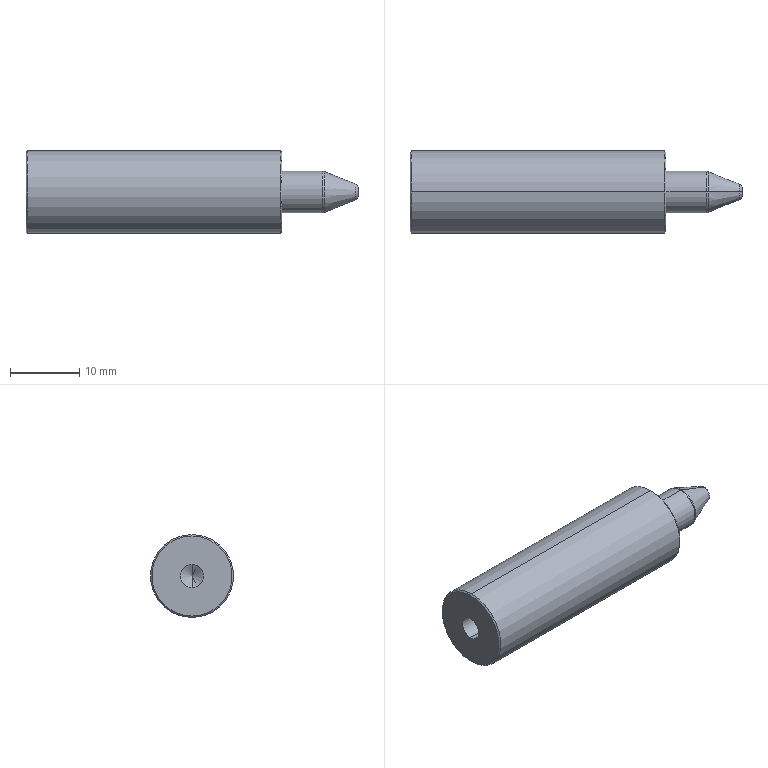Part | STEP file | 1 solid | 21 faces | box 48 x 12 x 12 mm | volume 4302 mm3 | cone 8 | cylinder 6 | torus 4 | plane 3 | commonest cylinder face diameters 3.3 x2 6 x2 12 x2
STEP:
#1=CARTESIAN_POINT('',(0.,0.,0.));
#2=DIRECTION('',(0.,0.,1.));
#3=DIRECTION('',(1.,0.,0.));
#4=AXIS2_PLACEMENT_3D('',#1,#2,#3);
#5=CARTESIAN_POINT('',(42.904,0.,3.));
#6=VERTEX_POINT('',#5);
#7=CARTESIAN_POINT('',(42.904,0.,-3.));
#8=VERTEX_POINT('',#7);
#9=CARTESIAN_POINT('',(42.904,0.,0.));
#10=DIRECTION('',(-1.,0.,0.));
#11=DIRECTION('',(0.,0.,-1.));
#12=AXIS2_PLACEMENT_3D('',#9,#10,#11);
#13=CIRCLE('',#12,3.);
#14=CARTESIAN_POINT('',(42.904,0.,0.));
#15=DIRECTION('',(1.,0.,0.));
#16=DIRECTION('',(0.,0.,-1.));
#17=AXIS2_PLACEMENT_3D('',#14,#15,#16);
#18=TOROIDAL_SURFACE('',#17,2.5,0.5);
#19=CARTESIAN_POINT('',(6.283,0.));
#20=DIRECTION('',(-1.,0.));
#21=VECTOR('',#20,1.);
#22=LINE('',#19,#21);
#23=(GEOMETRIC_REPRESENTATION_CONTEXT(2)PARAMETRIC_REPRESENTATION_CONTEXT()REPRESENTATION_CONTEXT('',''));
#24=DEFINITIONAL_REPRESENTATION('',(#22),#23);
#25=PCURVE('',#18,#24);
#26=CARTESIAN_POINT('',(0.,0.,0.));
#27=DIRECTION('',(-1.,0.,0.));
#28=DIRECTION('',(0.,0.,1.));
#29=AXIS2_PLACEMENT_3D('',#26,#27,#28);
#30=CYLINDRICAL_SURFACE('',#29,3.);
#31=CARTESIAN_POINT('',(-3.142,-42.904));
#32=DIRECTION('',(1.,0.));
#33=VECTOR('',#32,1.);
#34=LINE('',#31,#33);
#35=(GEOMETRIC_REPRESENTATION_CONTEXT(2)PARAMETRIC_REPRESENTATION_CONTEXT()REPRESENTATION_CONTEXT('',''));
#36=DEFINITIONAL_REPRESENTATION('',(#34),#35);
#37=PCURVE('',#30,#36);
#38=SURFACE_CURVE('',#13,(#25,#37),.PCURVE_S1.);
#39=EDGE_CURVE('',#6,#8,#38,.T.);
#40=ORIENTED_EDGE('',*,*,#39,.F.);
#41=CARTESIAN_POINT('',(43.089,0.,2.964));
#42=VERTEX_POINT('',#41);
#43=CARTESIAN_POINT('',(42.904,0.,2.5));
#44=DIRECTION('',(0.,1.,0.));
#45=DIRECTION('',(0.,0.,1.));
#46=AXIS2_PLACEMENT_3D('',#43,#44,#45);
#47=CIRCLE('',#46,0.5);
#48=CARTESIAN_POINT('',(3.142,0.));
#49=DIRECTION('',(0.,1.));
#50=VECTOR('',#49,1.);
#51=LINE('',#48,#50);
#52=(GEOMETRIC_REPRESENTATION_CONTEXT(2)PARAMETRIC_REPRESENTATION_CONTEXT()REPRESENTATION_CONTEXT('',''));
#53=DEFINITIONAL_REPRESENTATION('',(#51),#52);
#54=PCURVE('',#18,#53);
#55=CARTESIAN_POINT('',(42.904,0.,0.));
#56=DIRECTION('',(1.,0.,0.));
#57=DIRECTION('',(0.,0.,-1.));
#58=AXIS2_PLACEMENT_3D('',#55,#56,#57);
#59=TOROIDAL_SURFACE('',#58,2.5,0.5);
#60=CARTESIAN_POINT('',(3.142,0.));
#61=DIRECTION('',(0.,1.));
#62=VECTOR('',#61,1.);
#63=LINE('',#60,#62);
#64=(GEOMETRIC_REPRESENTATION_CONTEXT(2)PARAMETRIC_REPRESENTATION_CONTEXT()REPRESENTATION_CONTEXT('',''));
#65=DEFINITIONAL_REPRESENTATION('',(#63),#64);
#66=PCURVE('',#59,#65);
#67=SURFACE_CURVE('',#47,(#54,#66),.PCURVE_S1.);
#68=EDGE_CURVE('',#6,#42,#67,.T.);
#69=ORIENTED_EDGE('',*,*,#68,.T.);
#70=CARTESIAN_POINT('',(43.089,0.,-2.964));
#71=VERTEX_POINT('',#70);
#72=CARTESIAN_POINT('',(43.089,0.,0.));
#73=DIRECTION('',(1.,0.,0.));
#74=DIRECTION('',(0.,0.,1.));
#75=AXIS2_PLACEMENT_3D('',#72,#73,#74);
#76=CIRCLE('',#75,2.964);
#77=CARTESIAN_POINT('',(-3.142,0.3805));
#78=DIRECTION('',(1.,0.));
#79=VECTOR('',#78,1.);
#80=LINE('',#77,#79);
#81=(GEOMETRIC_REPRESENTATION_CONTEXT(2)PARAMETRIC_REPRESENTATION_CONTEXT()REPRESENTATION_CONTEXT('',''));
#82=DEFINITIONAL_REPRESENTATION('',(#80),#81);
#83=PCURVE('',#18,#82);
#84=CARTESIAN_POINT('',(43.,0.,0.));
#85=DIRECTION('',(-1.,0.,0.));
#86=DIRECTION('',(0.,0.,1.));
#87=AXIS2_PLACEMENT_3D('',#84,#85,#86);
#88=CONICAL_SURFACE('',#87,3.,0.3805);
#89=CARTESIAN_POINT('',(6.283,-0.0894));
#90=DIRECTION('',(-1.,0.));
#91=VECTOR('',#90,1.);
#92=LINE('',#89,#91);
#93=(GEOMETRIC_REPRESENTATION_CONTEXT(2)PARAMETRIC_REPRESENTATION_CONTEXT()REPRESENTATION_CONTEXT('',''));
#94=DEFINITIONAL_REPRESENTATION('',(#92),#93);
#95=PCURVE('',#88,#94);
#96=SURFACE_CURVE('',#76,(#83,#95),.PCURVE_S1.);
#97=EDGE_CURVE('',#71,#42,#96,.T.);
#98=ORIENTED_EDGE('',*,*,#97,.F.);
#99=CARTESIAN_POINT('',(42.904,0.,-2.5));
#100=DIRECTION('',(0.,-1.,0.));
#101=DIRECTION('',(0.,0.,-1.));
#102=AXIS2_PLACEMENT_3D('',#99,#100,#101);
#103=CIRCLE('',#102,0.5);
#104=CARTESIAN_POINT('',(0.,0.));
#105=DIRECTION('',(0.,1.));
#106=VECTOR('',#105,1.);
#107=LINE('',#104,#106);
#108=(GEOMETRIC_REPRESENTATION_CONTEXT(2)PARAMETRIC_REPRESENTATION_CONTEXT()REPRESENTATION_CONTEXT('',''));
#109=DEFINITIONAL_REPRESENTATION('',(#107),#108);
#110=PCURVE('',#18,#109);
#111=CARTESIAN_POINT('',(6.283,0.));
#112=DIRECTION('',(0.,1.));
#113=VECTOR('',#112,1.);
#114=LINE('',#111,#113);
#115=(GEOMETRIC_REPRESENTATION_CONTEXT(2)PARAMETRIC_REPRESENTATION_CONTEXT()REPRESENTATION_CONTEXT('',''));
#116=DEFINITIONAL_REPRESENTATION('',(#114),#115);
#117=PCURVE('',#59,#116);
#118=SURFACE_CURVE('',#103,(#110,#117),.PCURVE_S1.);
#119=EDGE_CURVE('',#8,#71,#118,.T.);
#120=ORIENTED_EDGE('',*,*,#119,.F.);
#121=EDGE_LOOP('',(#40,#69,#98,#120));
#122=FACE_BOUND('',#121,.T.);
#123=ADVANCED_FACE('',(#122),#18,.T.);
#124=CARTESIAN_POINT('',(48.,0.,-0.6615));
#125=VERTEX_POINT('',#124);
#126=CARTESIAN_POINT('',(48.,0.,0.6615));
#127=VERTEX_POINT('',#126);
#128=CARTESIAN_POINT('',(48.,0.,0.));
#129=DIRECTION('',(1.,0.,0.));
#130=DIRECTION('',(0.,0.,1.));
#131=AXIS2_PLACEMENT_3D('',#128,#129,#130);
#132=CIRCLE('',#131,0.6615);
#133=CARTESIAN_POINT('',(47.5,0.,0.));
#134=DIRECTION('',(-1.,0.,0.));
#135=DIRECTION('',(0.,0.,1.));
#136=AXIS2_PLACEMENT_3D('',#133,#134,#135);
#137=TOROIDAL_SURFACE('',#136,0.6615,0.5);
#138=CARTESIAN_POINT('',(6.283,4.712));
#139=DIRECTION('',(-1.,0.));
#140=VECTOR('',#139,1.);
#141=LINE('',#138,#140);
#142=(GEOMETRIC_REPRESENTATION_CONTEXT(2)PARAMETRIC_REPRESENTATION_CONTEXT()REPRESENTATION_CONTEXT('',''));
#143=DEFINITIONAL_REPRESENTATION('',(#141),#142);
#144=PCURVE('',#137,#143);
#145=CARTESIAN_POINT('',(48.,0.,0.));
#146=DIRECTION('',(-1.,0.,0.));
#147=DIRECTION('',(0.,0.,1.));
#148=AXIS2_PLACEMENT_3D('',#145,#146,#147);
#149=PLANE('',#148);
#150=CARTESIAN_POINT('',(0.6615,0.));
#151=CARTESIAN_POINT('',(0.6615,-1.146));
#152=CARTESIAN_POINT('',(-0.3307,-0.5729));
#153=CARTESIAN_POINT('',(-1.323,0.));
#154=CARTESIAN_POINT('',(-0.3307,0.5729));
#155=CARTESIAN_POINT('',(0.6615,1.146));
#156=CARTESIAN_POINT('',(0.6615,0.));
#157=(BOUNDED_CURVE()B_SPLINE_CURVE(2,(#150,#151,#152,#153,#154,#155,#156),.UNSPECIFIED.,.T.,.F.)B_SPLINE_CURVE_WITH_KNOTS((1,2,2,2,2,1),(-2.094,0.,2.094,4.189,6.283,8.378),.UNSPECIFIED.)CURVE()GEOMETRIC_REPRESENTATION_ITEM()RATIONAL_B_SPLINE_CURVE((1.,0.5,1.,0.5,1.,0.5,1.))REPRESENTATION_ITEM(''));
#158=(GEOMETRIC_REPRESENTATION_CONTEXT(2)PARAMETRIC_REPRESENTATION_CONTEXT()REPRESENTATION_CONTEXT('',''));
#159=DEFINITIONAL_REPRESENTATION('',(#157),#158);
#160=PCURVE('',#149,#159);
#161=SURFACE_CURVE('',#132,(#144,#160),.PCURVE_S1.);
#162=EDGE_CURVE('',#125,#127,#161,.T.);
#163=ORIENTED_EDGE('',*,*,#162,.F.);
#164=CARTESIAN_POINT('',(47.686,0.,-1.126));
#165=VERTEX_POINT('',#164);
#166=CARTESIAN_POINT('',(47.5,0.,-0.6615));
#167=DIRECTION('',(0.,1.,0.));
#168=DIRECTION('',(0.,0.,1.));
#169=AXIS2_PLACEMENT_3D('',#166,#167,#168);
#170=CIRCLE('',#169,0.5);
#171=CARTESIAN_POINT('',(3.142,3.142));
#172=DIRECTION('',(0.,1.));
#173=VECTOR('',#172,1.);
#174=LINE('',#171,#173);
#175=(GEOMETRIC_REPRESENTATION_CONTEXT(2)PARAMETRIC_REPRESENTATION_CONTEXT()REPRESENTATION_CONTEXT('',''));
#176=DEFINITIONAL_REPRESENTATION('',(#174),#175);
#177=PCURVE('',#137,#176);
#178=CARTESIAN_POINT('',(47.5,0.,0.));
#179=DIRECTION('',(-1.,0.,0.));
#180=DIRECTION('',(0.,0.,1.));
#181=AXIS2_PLACEMENT_3D('',#178,#179,#180);
#182=TOROIDAL_SURFACE('',#181,0.6615,0.5);
#183=CARTESIAN_POINT('',(3.142,3.142));
#184=DIRECTION('',(0.,1.));
#185=VECTOR('',#184,1.);
#186=LINE('',#183,#185);
#187=(GEOMETRIC_REPRESENTATION_CONTEXT(2)PARAMETRIC_REPRESENTATION_CONTEXT()REPRESENTATION_CONTEXT('',''));
#188=DEFINITIONAL_REPRESENTATION('',(#186),#187);
#189=PCURVE('',#182,#188);
#190=SURFACE_CURVE('',#170,(#177,#189),.PCURVE_S1.);
#191=EDGE_CURVE('',#125,#165,#190,.T.);
#192=ORIENTED_EDGE('',*,*,#191,.T.);
#193=CARTESIAN_POINT('',(47.686,0.,1.126));
#194=VERTEX_POINT('',#193);
#195=CARTESIAN_POINT('',(47.686,0.,0.));
#196=DIRECTION('',(-1.,0.,0.));
#197=DIRECTION('',(0.,0.,1.));
#198=AXIS2_PLACEMENT_3D('',#195,#196,#197);
#199=CIRCLE('',#198,1.126);
#200=CARTESIAN_POINT('',(0.,5.903));
#201=DIRECTION('',(1.,0.));
#202=VECTOR('',#201,1.);
#203=LINE('',#200,#202);
#204=(GEOMETRIC_REPRESENTATION_CONTEXT(2)PARAMETRIC_REPRESENTATION_CONTEXT()REPRESENTATION_CONTEXT('',''));
#205=DEFINITIONAL_REPRESENTATION('',(#203),#204);
#206=PCURVE('',#137,#205);
#207=CARTESIAN_POINT('',(0.,-4.686));
#208=DIRECTION('',(1.,0.));
#209=VECTOR('',#208,1.);
#210=LINE('',#207,#209);
#211=(GEOMETRIC_REPRESENTATION_CONTEXT(2)PARAMETRIC_REPRESENTATION_CONTEXT()REPRESENTATION_CONTEXT('',''));
#212=DEFINITIONAL_REPRESENTATION('',(#210),#211);
#213=PCURVE('',#88,#212);
#214=SURFACE_CURVE('',#199,(#206,#213),.PCURVE_S1.);
#215=EDGE_CURVE('',#194,#165,#214,.T.);
#216=ORIENTED_EDGE('',*,*,#215,.F.);
#217=CARTESIAN_POINT('',(47.5,0.,0.6615));
#218=DIRECTION('',(0.,-1.,0.));
#219=DIRECTION('',(0.,0.,-1.));
#220=AXIS2_PLACEMENT_3D('',#217,#218,#219);
#221=CIRCLE('',#220,0.5);
#222=CARTESIAN_POINT('',(0.,3.142));
#223=DIRECTION('',(0.,1.));
#224=VECTOR('',#223,1.);
#225=LINE('',#222,#224);
#226=(GEOMETRIC_REPRESENTATION_CONTEXT(2)PARAMETRIC_REPRESENTATION_CONTEXT()REPRESENTATION_CONTEXT('',''));
#227=DEFINITIONAL_REPRESENTATION('',(#225),#226);
#228=PCURVE('',#137,#227);
#229=CARTESIAN_POINT('',(6.283,3.142));
#230=DIRECTION('',(0.,1.));
#231=VECTOR('',#230,1.);
#232=LINE('',#229,#231);
#233=(GEOMETRIC_REPRESENTATION_CONTEXT(2)PARAMETRIC_REPRESENTATION_CONTEXT()REPRESENTATION_CONTEXT('',''));
#234=DEFINITIONAL_REPRESENTATION('',(#232),#233);
#235=PCURVE('',#182,#234);
#236=SURFACE_CURVE('',#221,(#228,#235),.PCURVE_S1.);
#237=EDGE_CURVE('',#127,#194,#236,.T.);
#238=ORIENTED_EDGE('',*,*,#237,.F.);
#239=EDGE_LOOP('',(#163,#192,#216,#238));
#240=FACE_BOUND('',#239,.T.);
#241=ADVANCED_FACE('',(#240),#137,.T.);
#242=CARTESIAN_POINT('',(0.,0.,5.8));
#243=VERTEX_POINT('',#242);
#244=CARTESIAN_POINT('',(0.,0.,-5.8));
#245=VERTEX_POINT('',#244);
#246=CARTESIAN_POINT('',(0.,0.,0.));
#247=DIRECTION('',(-1.,0.,0.));
#248=DIRECTION('',(0.,0.,-1.));
#249=AXIS2_PLACEMENT_3D('',#246,#247,#248);
#250=CIRCLE('',#249,5.8);
#251=CARTESIAN_POINT('',(0.,0.,0.));
#252=DIRECTION('',(1.,0.,0.));
#253=DIRECTION('',(0.,0.,-1.));
#254=AXIS2_PLACEMENT_3D('',#251,#252,#253);
#255=CONICAL_SURFACE('',#254,5.8,0.7854);
#256=CARTESIAN_POINT('',(6.283,0.));
#257=DIRECTION('',(-1.,0.));
#258=VECTOR('',#257,1.);
#259=LINE('',#256,#258);
#260=(GEOMETRIC_REPRESENTATION_CONTEXT(2)PARAMETRIC_REPRESENTATION_CONTEXT()REPRESENTATION_CONTEXT('',''));
#261=DEFINITIONAL_REPRESENTATION('',(#259),#260);
#262=PCURVE('',#255,#261);
#263=CARTESIAN_POINT('',(0.,6.,0.));
#264=DIRECTION('',(1.,0.,0.));
#265=DIRECTION('',(0.,0.,-1.));
#266=AXIS2_PLACEMENT_3D('',#263,#264,#265);
#267=PLANE('',#266);
#268=CARTESIAN_POINT('',(5.8,-6.));
#269=CARTESIAN_POINT('',(5.8,-16.046));
#270=CARTESIAN_POINT('',(-2.9,-11.023));
#271=CARTESIAN_POINT('',(-11.6,-6.));
#272=CARTESIAN_POINT('',(-2.9,-0.9771));
#273=CARTESIAN_POINT('',(5.8,4.046));
#274=CARTESIAN_POINT('',(5.8,-6.));
#275=(BOUNDED_CURVE()B_SPLINE_CURVE(2,(#268,#269,#270,#271,#272,#273,#274),.UNSPECIFIED.,.T.,.F.)B_SPLINE_CURVE_WITH_KNOTS((1,2,2,2,2,1),(-2.094,0.,2.094,4.189,6.283,8.378),.UNSPECIFIED.)CURVE()GEOMETRIC_REPRESENTATION_ITEM()RATIONAL_B_SPLINE_CURVE((1.,0.5,1.,0.5,1.,0.5,1.))REPRESENTATION_ITEM(''));
#276=(GEOMETRIC_REPRESENTATION_CONTEXT(2)PARAMETRIC_REPRESENTATION_CONTEXT()REPRESENTATION_CONTEXT('',''));
#277=DEFINITIONAL_REPRESENTATION('',(#275),#276);
#278=PCURVE('',#267,#277);
#279=SURFACE_CURVE('',#250,(#262,#278),.PCURVE_S1.);
#280=EDGE_CURVE('',#243,#245,#279,.T.);
#281=ORIENTED_EDGE('',*,*,#280,.F.);
#282=CARTESIAN_POINT('',(0.2,0.,6.));
#283=VERTEX_POINT('',#282);
#284=CARTESIAN_POINT('',(0.,0.,5.8));
#285=DIRECTION('',(0.7071,0.,0.7071));
#286=VECTOR('',#285,1.);
#287=LINE('',#284,#286);
#288=CARTESIAN_POINT('',(3.142,0.));
#289=DIRECTION('',(0.,1.));
#290=VECTOR('',#289,1.);
#291=LINE('',#288,#290);
#292=(GEOMETRIC_REPRESENTATION_CONTEXT(2)PARAMETRIC_REPRESENTATION_CONTEXT()REPRESENTATION_CONTEXT('',''));
#293=DEFINITIONAL_REPRESENTATION('',(#291),#292);
#294=PCURVE('',#255,#293);
#295=CARTESIAN_POINT('',(0.,0.,0.));
#296=DIRECTION('',(1.,0.,0.));
#297=DIRECTION('',(0.,0.,-1.));
#298=AXIS2_PLACEMENT_3D('',#295,#296,#297);
#299=CONICAL_SURFACE('',#298,5.8,0.7854);
#300=CARTESIAN_POINT('',(3.142,0.));
#301=DIRECTION('',(0.,1.));
#302=VECTOR('',#301,1.);
#303=LINE('',#300,#302);
#304=(GEOMETRIC_REPRESENTATION_CONTEXT(2)PARAMETRIC_REPRESENTATION_CONTEXT()REPRESENTATION_CONTEXT('',''));
#305=DEFINITIONAL_REPRESENTATION('',(#303),#304);
#306=PCURVE('',#299,#305);
#307=SURFACE_CURVE('',#287,(#294,#306),.PCURVE_S1.);
#308=EDGE_CURVE('',#243,#283,#307,.T.);
#309=ORIENTED_EDGE('',*,*,#308,.T.);
#310=CARTESIAN_POINT('',(0.2,0.,-6.));
#311=VERTEX_POINT('',#310);
#312=CARTESIAN_POINT('',(0.2,0.,0.));
#313=DIRECTION('',(1.,0.,0.));
#314=DIRECTION('',(0.,0.,-1.));
#315=AXIS2_PLACEMENT_3D('',#312,#313,#314);
#316=CIRCLE('',#315,6.);
#317=CARTESIAN_POINT('',(0.,0.2));
#318=DIRECTION('',(1.,0.));
#319=VECTOR('',#318,1.);
#320=LINE('',#317,#319);
#321=(GEOMETRIC_REPRESENTATION_CONTEXT(2)PARAMETRIC_REPRESENTATION_CONTEXT()REPRESENTATION_CONTEXT('',''));
#322=DEFINITIONAL_REPRESENTATION('',(#320),#321);
#323=PCURVE('',#255,#322);
#324=CARTESIAN_POINT('',(0.,0.,0.));
#325=DIRECTION('',(-1.,0.,0.));
#326=DIRECTION('',(0.,0.,1.));
#327=AXIS2_PLACEMENT_3D('',#324,#325,#326);
#328=CYLINDRICAL_SURFACE('',#327,6.);
#329=CARTESIAN_POINT('',(3.142,-0.2));
#330=DIRECTION('',(-1.,0.));
#331=VECTOR('',#330,1.);
#332=LINE('',#329,#331);
#333=(GEOMETRIC_REPRESENTATION_CONTEXT(2)PARAMETRIC_REPRESENTATION_CONTEXT()REPRESENTATION_CONTEXT('',''));
#334=DEFINITIONAL_REPRESENTATION('',(#332),#333);
#335=PCURVE('',#328,#334);
#336=SURFACE_CURVE('',#316,(#323,#335),.PCURVE_S1.);
#337=EDGE_CURVE('',#311,#283,#336,.T.);
#338=ORIENTED_EDGE('',*,*,#337,.F.);
#339=CARTESIAN_POINT('',(0.,0.,-5.8));
#340=DIRECTION('',(0.7071,0.,-0.7071));
#341=VECTOR('',#340,1.);
#342=LINE('',#339,#341);
#343=CARTESIAN_POINT('',(0.,0.));
#344=DIRECTION('',(0.,1.));
#345=VECTOR('',#344,1.);
#346=LINE('',#343,#345);
#347=(GEOMETRIC_REPRESENTATION_CONTEXT(2)PARAMETRIC_REPRESENTATION_CONTEXT()REPRESENTATION_CONTEXT('',''));
#348=DEFINITIONAL_REPRESENTATION('',(#346),#347);
#349=PCURVE('',#255,#348);
#350=CARTESIAN_POINT('',(6.283,0.));
#351=DIRECTION('',(0.,1.));
#352=VECTOR('',#351,1.);
#353=LINE('',#350,#352);
#354=(GEOMETRIC_REPRESENTATION_CONTEXT(2)PARAMETRIC_REPRESENTATION_CONTEXT()REPRESENTATION_CONTEXT('',''));
#355=DEFINITIONAL_REPRESENTATION('',(#353),#354);
#356=PCURVE('',#299,#355);
#357=SURFACE_CURVE('',#342,(#349,#356),.PCURVE_S1.);
#358=EDGE_CURVE('',#245,#311,#357,.T.);
#359=ORIENTED_EDGE('',*,*,#358,.F.);
#360=EDGE_LOOP('',(#281,#309,#338,#359));
#361=FACE_BOUND('',#360,.T.);
#362=ADVANCED_FACE('',(#361),#255,.T.);
#363=CARTESIAN_POINT('',(37.,0.,-5.8));
#364=VERTEX_POINT('',#363);
#365=CARTESIAN_POINT('',(37.,0.,5.8));
#366=VERTEX_POINT('',#365);
#367=CARTESIAN_POINT('',(37.,0.,0.));
#368=DIRECTION('',(1.,0.,0.));
#369=DIRECTION('',(0.,0.,1.));
#370=AXIS2_PLACEMENT_3D('',#367,#368,#369);
#371=CIRCLE('',#370,5.8);
#372=CARTESIAN_POINT('',(36.8,0.,0.));
#373=DIRECTION('',(-1.,0.,0.));
#374=DIRECTION('',(0.,0.,1.));
#375=AXIS2_PLACEMENT_3D('',#372,#373,#374);
#376=CONICAL_SURFACE('',#375,6.,0.7854);
#377=CARTESIAN_POINT('',(6.283,-0.2));
#378=DIRECTION('',(-1.,0.));
#379=VECTOR('',#378,1.);
#380=LINE('',#377,#379);
#381=(GEOMETRIC_REPRESENTATION_CONTEXT(2)PARAMETRIC_REPRESENTATION_CONTEXT()REPRESENTATION_CONTEXT('',''));
#382=DEFINITIONAL_REPRESENTATION('',(#380),#381);
#383=PCURVE('',#376,#382);
#384=CARTESIAN_POINT('',(37.,3.,0.));
#385=DIRECTION('',(-1.,0.,0.));
#386=DIRECTION('',(0.,0.,1.));
#387=AXIS2_PLACEMENT_3D('',#384,#385,#386);
#388=PLANE('',#387);
#389=CARTESIAN_POINT('',(5.8,-3.));
#390=CARTESIAN_POINT('',(5.8,-13.046));
#391=CARTESIAN_POINT('',(-2.9,-8.023));
#392=CARTESIAN_POINT('',(-11.6,-3.));
#393=CARTESIAN_POINT('',(-2.9,2.023));
#394=CARTESIAN_POINT('',(5.8,7.046));
#395=CARTESIAN_POINT('',(5.8,-3.));
#396=(BOUNDED_CURVE()B_SPLINE_CURVE(2,(#389,#390,#391,#392,#393,#394,#395),.UNSPECIFIED.,.T.,.F.)B_SPLINE_CURVE_WITH_KNOTS((1,2,2,2,2,1),(-2.094,0.,2.094,4.189,6.283,8.378),.UNSPECIFIED.)CURVE()GEOMETRIC_REPRESENTATION_ITEM()RATIONAL_B_SPLINE_CURVE((1.,0.5,1.,0.5,1.,0.5,1.))REPRESENTATION_ITEM(''));
#397=(GEOMETRIC_REPRESENTATION_CONTEXT(2)PARAMETRIC_REPRESENTATION_CONTEXT()REPRESENTATION_CONTEXT('',''));
#398=DEFINITIONAL_REPRESENTATION('',(#396),#397);
#399=PCURVE('',#388,#398);
#400=SURFACE_CURVE('',#371,(#383,#399),.PCURVE_S1.);
#401=EDGE_CURVE('',#364,#366,#400,.T.);
#402=ORIENTED_EDGE('',*,*,#401,.F.);
#403=CARTESIAN_POINT('',(36.8,0.,-6.));
#404=VERTEX_POINT('',#403);
#405=CARTESIAN_POINT('',(36.8,0.,-6.));
#406=DIRECTION('',(-0.7071,0.,-0.7071));
#407=VECTOR('',#406,1.);
#408=LINE('',#405,#407);
#409=CARTESIAN_POINT('',(3.142,0.));
#410=DIRECTION('',(0.,1.));
#411=VECTOR('',#410,1.);
#412=LINE('',#409,#411);
#413=(GEOMETRIC_REPRESENTATION_CONTEXT(2)PARAMETRIC_REPRESENTATION_CONTEXT()REPRESENTATION_CONTEXT('',''));
#414=DEFINITIONAL_REPRESENTATION('',(#412),#413);
#415=PCURVE('',#376,#414);
#416=CARTESIAN_POINT('',(36.8,0.,0.));
#417=DIRECTION('',(-1.,0.,0.));
#418=DIRECTION('',(0.,0.,1.));
#419=AXIS2_PLACEMENT_3D('',#416,#417,#418);
#420=CONICAL_SURFACE('',#419,6.,0.7854);
#421=CARTESIAN_POINT('',(3.142,0.));
#422=DIRECTION('',(0.,1.));
#423=VECTOR('',#422,1.);
#424=LINE('',#421,#423);
#425=(GEOMETRIC_REPRESENTATION_CONTEXT(2)PARAMETRIC_REPRESENTATION_CONTEXT()REPRESENTATION_CONTEXT('',''));
#426=DEFINITIONAL_REPRESENTATION('',(#424),#425);
#427=PCURVE('',#420,#426);
#428=SURFACE_CURVE('',#408,(#415,#427),.PCURVE_S1.);
#429=EDGE_CURVE('',#364,#404,#428,.T.);
#430=ORIENTED_EDGE('',*,*,#429,.T.);
#431=CARTESIAN_POINT('',(36.8,0.,6.));
#432=VERTEX_POINT('',#431);
#433=CARTESIAN_POINT('',(36.8,0.,0.));
#434=DIRECTION('',(-1.,0.,0.));
#435=DIRECTION('',(0.,0.,1.));
#436=AXIS2_PLACEMENT_3D('',#433,#434,#435);
#437=CIRCLE('',#436,6.);
#438=CARTESIAN_POINT('',(0.,0.));
#439=DIRECTION('',(1.,0.));
#440=VECTOR('',#439,1.);
#441=LINE('',#438,#440);
#442=(GEOMETRIC_REPRESENTATION_CONTEXT(2)PARAMETRIC_REPRESENTATION_CONTEXT()REPRESENTATION_CONTEXT('',''));
#443=DEFINITIONAL_REPRESENTATION('',(#441),#442);
#444=PCURVE('',#376,#443);
#445=CARTESIAN_POINT('',(0.,-36.8));
#446=DIRECTION('',(1.,0.));
#447=VECTOR('',#446,1.);
#448=LINE('',#445,#447);
#449=(GEOMETRIC_REPRESENTATION_CONTEXT(2)PARAMETRIC_REPRESENTATION_CONTEXT()REPRESENTATION_CONTEXT('',''));
#450=DEFINITIONAL_REPRESENTATION('',(#448),#449);
#451=PCURVE('',#328,#450);
#452=SURFACE_CURVE('',#437,(#444,#451),.PCURVE_S1.);
#453=EDGE_CURVE('',#432,#404,#452,.T.);
#454=ORIENTED_EDGE('',*,*,#453,.F.);
#455=CARTESIAN_POINT('',(36.8,0.,6.));
#456=DIRECTION('',(-0.7071,0.,0.7071));
#457=VECTOR('',#456,1.);
#458=LINE('',#455,#457);
#459=CARTESIAN_POINT('',(0.,0.));
#460=DIRECTION('',(0.,1.));
#461=VECTOR('',#460,1.);
#462=LINE('',#459,#461);
#463=(GEOMETRIC_REPRESENTATION_CONTEXT(2)PARAMETRIC_REPRESENTATION_CONTEXT()REPRESENTATION_CONTEXT('',''));
#464=DEFINITIONAL_REPRESENTATION('',(#462),#463);
#465=PCURVE('',#376,#464);
#466=CARTESIAN_POINT('',(6.283,0.));
#467=DIRECTION('',(0.,1.));
#468=VECTOR('',#467,1.);
#469=LINE('',#466,#468);
#470=(GEOMETRIC_REPRESENTATION_CONTEXT(2)PARAMETRIC_REPRESENTATION_CONTEXT()REPRESENTATION_CONTEXT('',''));
#471=DEFINITIONAL_REPRESENTATION('',(#469),#470);
#472=PCURVE('',#420,#471);
#473=SURFACE_CURVE('',#458,(#465,#472),.PCURVE_S1.);
#474=EDGE_CURVE('',#366,#432,#473,.T.);
#475=ORIENTED_EDGE('',*,*,#474,.F.);
#476=EDGE_LOOP('',(#402,#430,#454,#475));
#477=FACE_BOUND('',#476,.T.);
#478=ADVANCED_FACE('',(#477),#376,.T.);
#479=ORIENTED_EDGE('',*,*,#215,.T.);
#480=CARTESIAN_POINT('',(43.,0.,-3.));
#481=DIRECTION('',(-0.9285,0.,-0.3714));
#482=VECTOR('',#481,1.);
#483=LINE('',#480,#482);
#484=CARTESIAN_POINT('',(3.142,0.));
#485=DIRECTION('',(0.,1.));
#486=VECTOR('',#485,1.);
#487=LINE('',#484,#486);
#488=(GEOMETRIC_REPRESENTATION_CONTEXT(2)PARAMETRIC_REPRESENTATION_CONTEXT()REPRESENTATION_CONTEXT('',''));
#489=DEFINITIONAL_REPRESENTATION('',(#487),#488);
#490=PCURVE('',#88,#489);
#491=CARTESIAN_POINT('',(43.,0.,0.));
#492=DIRECTION('',(-1.,0.,0.));
#493=DIRECTION('',(0.,0.,1.));
#494=AXIS2_PLACEMENT_3D('',#491,#492,#493);
#495=CONICAL_SURFACE('',#494,3.,0.3805);
#496=CARTESIAN_POINT('',(3.142,0.));
#497=DIRECTION('',(0.,1.));
#498=VECTOR('',#497,1.);
#499=LINE('',#496,#498);
#500=(GEOMETRIC_REPRESENTATION_CONTEXT(2)PARAMETRIC_REPRESENTATION_CONTEXT()REPRESENTATION_CONTEXT('',''));
#501=DEFINITIONAL_REPRESENTATION('',(#499),#500);
#502=PCURVE('',#495,#501);
#503=SURFACE_CURVE('',#483,(#490,#502),.PCURVE_S1.);
#504=EDGE_CURVE('',#165,#71,#503,.T.);
#505=ORIENTED_EDGE('',*,*,#504,.T.);
#506=ORIENTED_EDGE('',*,*,#97,.T.);
#507=CARTESIAN_POINT('',(43.,0.,3.));
#508=DIRECTION('',(-0.9285,0.,0.3714));
#509=VECTOR('',#508,1.);
#510=LINE('',#507,#509);
#511=CARTESIAN_POINT('',(0.,0.));
#512=DIRECTION('',(0.,1.));
#513=VECTOR('',#512,1.);
#514=LINE('',#511,#513);
#515=(GEOMETRIC_REPRESENTATION_CONTEXT(2)PARAMETRIC_REPRESENTATION_CONTEXT()REPRESENTATION_CONTEXT('',''));
#516=DEFINITIONAL_REPRESENTATION('',(#514),#515);
#517=PCURVE('',#88,#516);
#518=CARTESIAN_POINT('',(6.283,0.));
#519=DIRECTION('',(0.,1.));
#520=VECTOR('',#519,1.);
#521=LINE('',#518,#520);
#522=(GEOMETRIC_REPRESENTATION_CONTEXT(2)PARAMETRIC_REPRESENTATION_CONTEXT()REPRESENTATION_CONTEXT('',''));
#523=DEFINITIONAL_REPRESENTATION('',(#521),#522);
#524=PCURVE('',#495,#523);
#525=SURFACE_CURVE('',#510,(#517,#524),.PCURVE_S1.);
#526=EDGE_CURVE('',#194,#42,#525,.T.);
#527=ORIENTED_EDGE('',*,*,#526,.F.);
#528=EDGE_LOOP('',(#479,#505,#506,#527));
#529=FACE_BOUND('',#528,.T.);
#530=ADVANCED_FACE('',(#529),#88,.T.);
#531=CARTESIAN_POINT('',(13.5,0.,1.65));
#532=VERTEX_POINT('',#531);
#533=CARTESIAN_POINT('',(0.,0.,1.65));
#534=VERTEX_POINT('',#533);
#535=CARTESIAN_POINT('',(0.,0.,1.65));
#536=DIRECTION('',(-1.,0.,0.));
#537=VECTOR('',#536,1.);
#538=LINE('',#535,#537);
#539=CARTESIAN_POINT('',(0.,0.,0.));
#540=DIRECTION('',(-1.,0.,0.));
#541=DIRECTION('',(0.,0.,1.));
#542=AXIS2_PLACEMENT_3D('',#539,#540,#541);
#543=CYLINDRICAL_SURFACE('',#542,1.65);
#544=CARTESIAN_POINT('',(6.283,0.));
#545=DIRECTION('',(0.,1.));
#546=VECTOR('',#545,1.);
#547=LINE('',#544,#546);
#548=(GEOMETRIC_REPRESENTATION_CONTEXT(2)PARAMETRIC_REPRESENTATION_CONTEXT()REPRESENTATION_CONTEXT('',''));
#549=DEFINITIONAL_REPRESENTATION('',(#547),#548);
#550=PCURVE('',#543,#549);
#551=CARTESIAN_POINT('',(0.,0.,0.));
#552=DIRECTION('',(-1.,0.,0.));
#553=DIRECTION('',(0.,0.,1.));
#554=AXIS2_PLACEMENT_3D('',#551,#552,#553);
#555=CYLINDRICAL_SURFACE('',#554,1.65);
#556=CARTESIAN_POINT('',(0.,0.));
#557=DIRECTION('',(0.,1.));
#558=VECTOR('',#557,1.);
#559=LINE('',#556,#558);
#560=(GEOMETRIC_REPRESENTATION_CONTEXT(2)PARAMETRIC_REPRESENTATION_CONTEXT()REPRESENTATION_CONTEXT('',''));
#561=DEFINITIONAL_REPRESENTATION('',(#559),#560);
#562=PCURVE('',#555,#561);
#563=SURFACE_CURVE('',#538,(#550,#562),.PCURVE_S1.);
#564=EDGE_CURVE('',#532,#534,#563,.T.);
#565=ORIENTED_EDGE('',*,*,#564,.T.);
#566=CARTESIAN_POINT('',(0.,0.,-1.65));
#567=VERTEX_POINT('',#566);
#568=CARTESIAN_POINT('',(0.,0.,0.));
#569=DIRECTION('',(-1.,0.,0.));
#570=DIRECTION('',(0.,0.,1.));
#571=AXIS2_PLACEMENT_3D('',#568,#569,#570);
#572=CIRCLE('',#571,1.65);
#573=CARTESIAN_POINT('',(0.,0.));
#574=DIRECTION('',(1.,0.));
#575=VECTOR('',#574,1.);
#576=LINE('',#573,#575);
#577=(GEOMETRIC_REPRESENTATION_CONTEXT(2)PARAMETRIC_REPRESENTATION_CONTEXT()REPRESENTATION_CONTEXT('',''));
#578=DEFINITIONAL_REPRESENTATION('',(#576),#577);
#579=PCURVE('',#543,#578);
#580=CARTESIAN_POINT('',(-1.65,-6.));
#581=CARTESIAN_POINT('',(-1.65,-3.142));
#582=CARTESIAN_POINT('',(0.825,-4.571));
#583=CARTESIAN_POINT('',(3.3,-6.));
#584=CARTESIAN_POINT('',(0.825,-7.429));
#585=CARTESIAN_POINT('',(-1.65,-8.858));
#586=CARTESIAN_POINT('',(-1.65,-6.));
#587=(BOUNDED_CURVE()B_SPLINE_CURVE(2,(#580,#581,#582,#583,#584,#585,#586),.UNSPECIFIED.,.T.,.F.)B_SPLINE_CURVE_WITH_KNOTS((1,2,2,2,2,1),(-2.094,0.,2.094,4.189,6.283,8.378),.UNSPECIFIED.)CURVE()GEOMETRIC_REPRESENTATION_ITEM()RATIONAL_B_SPLINE_CURVE((1.,0.5,1.,0.5,1.,0.5,1.))REPRESENTATION_ITEM(''));
#588=(GEOMETRIC_REPRESENTATION_CONTEXT(2)PARAMETRIC_REPRESENTATION_CONTEXT()REPRESENTATION_CONTEXT('',''));
#589=DEFINITIONAL_REPRESENTATION('',(#587),#588);
#590=PCURVE('',#267,#589);
#591=SURFACE_CURVE('',#572,(#579,#590),.PCURVE_S1.);
#592=EDGE_CURVE('',#567,#534,#591,.T.);
#593=ORIENTED_EDGE('',*,*,#592,.F.);
#594=CARTESIAN_POINT('',(13.5,0.,-1.65));
#595=VERTEX_POINT('',#594);
#596=CARTESIAN_POINT('',(0.,0.,-1.65));
#597=DIRECTION('',(-1.,0.,0.));
#598=VECTOR('',#597,1.);
#599=LINE('',#596,#598);
#600=CARTESIAN_POINT('',(3.142,0.));
#601=DIRECTION('',(0.,1.));
#602=VECTOR('',#601,1.);
#603=LINE('',#600,#602);
#604=(GEOMETRIC_REPRESENTATION_CONTEXT(2)PARAMETRIC_REPRESENTATION_CONTEXT()REPRESENTATION_CONTEXT('',''));
#605=DEFINITIONAL_REPRESENTATION('',(#603),#604);
#606=PCURVE('',#543,#605);
#607=CARTESIAN_POINT('',(3.142,0.));
#608=DIRECTION('',(0.,1.));
#609=VECTOR('',#608,1.);
#610=LINE('',#607,#609);
#611=(GEOMETRIC_REPRESENTATION_CONTEXT(2)PARAMETRIC_REPRESENTATION_CONTEXT()REPRESENTATION_CONTEXT('',''));
#612=DEFINITIONAL_REPRESENTATION('',(#610),#611);
#613=PCURVE('',#555,#612);
#614=SURFACE_CURVE('',#599,(#606,#613),.PCURVE_S1.);
#615=EDGE_CURVE('',#595,#567,#614,.T.);
#616=ORIENTED_EDGE('',*,*,#615,.F.);
#617=CARTESIAN_POINT('',(13.5,0.,0.));
#618=DIRECTION('',(-1.,0.,0.));
#619=DIRECTION('',(0.,0.,1.));
#620=AXIS2_PLACEMENT_3D('',#617,#618,#619);
#621=CIRCLE('',#620,1.65);
#622=CARTESIAN_POINT('',(0.,-13.5));
#623=DIRECTION('',(1.,0.));
#624=VECTOR('',#623,1.);
#625=LINE('',#622,#624);
#626=(GEOMETRIC_REPRESENTATION_CONTEXT(2)PARAMETRIC_REPRESENTATION_CONTEXT()REPRESENTATION_CONTEXT('',''));
#627=DEFINITIONAL_REPRESENTATION('',(#625),#626);
#628=PCURVE('',#543,#627);
#629=CARTESIAN_POINT('',(13.5,0.,0.));
#630=DIRECTION('',(-1.,0.,0.));
#631=DIRECTION('',(0.,0.,1.));
#632=AXIS2_PLACEMENT_3D('',#629,#630,#631);
#633=CONICAL_SURFACE('',#632,1.65,1.03);
#634=CARTESIAN_POINT('',(0.,0.));
#635=DIRECTION('',(1.,0.));
#636=VECTOR('',#635,1.);
#637=LINE('',#634,#636);
#638=(GEOMETRIC_REPRESENTATION_CONTEXT(2)PARAMETRIC_REPRESENTATION_CONTEXT()REPRESENTATION_CONTEXT('',''));
#639=DEFINITIONAL_REPRESENTATION('',(#637),#638);
#640=PCURVE('',#633,#639);
#641=SURFACE_CURVE('',#621,(#628,#640),.PCURVE_S1.);
#642=EDGE_CURVE('',#595,#532,#641,.T.);
#643=ORIENTED_EDGE('',*,*,#642,.T.);
#644=EDGE_LOOP('',(#565,#593,#616,#643));
#645=FACE_BOUND('',#644,.F.);
#646=ADVANCED_FACE('',(#645),#543,.F.);
#647=ORIENTED_EDGE('',*,*,#642,.F.);
#648=CARTESIAN_POINT('',(14.491,0.,0.));
#649=VERTEX_POINT('',#648);
#650=CARTESIAN_POINT('',(13.5,0.,-1.65));
#651=DIRECTION('',(-0.515,0.,-0.8572));
#652=VECTOR('',#651,1.);
#653=LINE('',#650,#652);
#654=CARTESIAN_POINT('',(3.142,0.));
#655=DIRECTION('',(0.,1.));
#656=VECTOR('',#655,1.);
#657=LINE('',#654,#656);
#658=(GEOMETRIC_REPRESENTATION_CONTEXT(2)PARAMETRIC_REPRESENTATION_CONTEXT()REPRESENTATION_CONTEXT('',''));
#659=DEFINITIONAL_REPRESENTATION('',(#657),#658);
#660=PCURVE('',#633,#659);
#661=CARTESIAN_POINT('',(13.5,0.,0.));
#662=DIRECTION('',(-1.,0.,0.));
#663=DIRECTION('',(0.,0.,1.));
#664=AXIS2_PLACEMENT_3D('',#661,#662,#663);
#665=CONICAL_SURFACE('',#664,1.65,1.03);
#666=CARTESIAN_POINT('',(3.142,0.));
#667=DIRECTION('',(0.,1.));
#668=VECTOR('',#667,1.);
#669=LINE('',#666,#668);
#670=(GEOMETRIC_REPRESENTATION_CONTEXT(2)PARAMETRIC_REPRESENTATION_CONTEXT()REPRESENTATION_CONTEXT('',''));
#671=DEFINITIONAL_REPRESENTATION('',(#669),#670);
#672=PCURVE('',#665,#671);
#673=SURFACE_CURVE('',#653,(#660,#672),.PCURVE_S1.);
#674=EDGE_CURVE('',#649,#595,#673,.T.);
#675=ORIENTED_EDGE('',*,*,#674,.F.);
#676=CARTESIAN_POINT('',(13.5,0.,1.65));
#677=DIRECTION('',(-0.515,0.,0.8572));
#678=VECTOR('',#677,1.);
#679=LINE('',#676,#678);
#680=CARTESIAN_POINT('',(6.283,0.));
#681=DIRECTION('',(0.,1.));
#682=VECTOR('',#681,1.);
#683=LINE('',#680,#682);
#684=(GEOMETRIC_REPRESENTATION_CONTEXT(2)PARAMETRIC_REPRESENTATION_CONTEXT()REPRESENTATION_CONTEXT('',''));
#685=DEFINITIONAL_REPRESENTATION('',(#683),#684);
#686=PCURVE('',#633,#685);
#687=CARTESIAN_POINT('',(0.,0.));
#688=DIRECTION('',(0.,1.));
#689=VECTOR('',#688,1.);
#690=LINE('',#687,#689);
#691=(GEOMETRIC_REPRESENTATION_CONTEXT(2)PARAMETRIC_REPRESENTATION_CONTEXT()REPRESENTATION_CONTEXT('',''));
#692=DEFINITIONAL_REPRESENTATION('',(#690),#691);
#693=PCURVE('',#665,#692);
#694=SURFACE_CURVE('',#679,(#686,#693),.PCURVE_S1.);
#695=EDGE_CURVE('',#649,#532,#694,.T.);
#696=ORIENTED_EDGE('',*,*,#695,.T.);
#697=EDGE_LOOP('',(#647,#675,#696));
#698=FACE_BOUND('',#697,.F.);
#699=ADVANCED_FACE('',(#698),#633,.F.);
#700=ORIENTED_EDGE('',*,*,#453,.T.);
#701=CARTESIAN_POINT('',(0.,0.,-6.));
#702=DIRECTION('',(-1.,0.,0.));
#703=VECTOR('',#702,1.);
#704=LINE('',#701,#703);
#705=CARTESIAN_POINT('',(3.142,0.));
#706=DIRECTION('',(0.,1.));
#707=VECTOR('',#706,1.);
#708=LINE('',#705,#707);
#709=(GEOMETRIC_REPRESENTATION_CONTEXT(2)PARAMETRIC_REPRESENTATION_CONTEXT()REPRESENTATION_CONTEXT('',''));
#710=DEFINITIONAL_REPRESENTATION('',(#708),#709);
#711=PCURVE('',#328,#710);
#712=CARTESIAN_POINT('',(0.,0.,0.));
#713=DIRECTION('',(-1.,0.,0.));
#714=DIRECTION('',(0.,0.,1.));
#715=AXIS2_PLACEMENT_3D('',#712,#713,#714);
#716=CYLINDRICAL_SURFACE('',#715,6.);
#717=CARTESIAN_POINT('',(3.142,0.));
#718=DIRECTION('',(0.,1.));
#719=VECTOR('',#718,1.);
#720=LINE('',#717,#719);
#721=(GEOMETRIC_REPRESENTATION_CONTEXT(2)PARAMETRIC_REPRESENTATION_CONTEXT()REPRESENTATION_CONTEXT('',''));
#722=DEFINITIONAL_REPRESENTATION('',(#720),#721);
#723=PCURVE('',#716,#722);
#724=SURFACE_CURVE('',#704,(#711,#723),.PCURVE_S1.);
#725=EDGE_CURVE('',#404,#311,#724,.T.);
#726=ORIENTED_EDGE('',*,*,#725,.T.);
#727=ORIENTED_EDGE('',*,*,#337,.T.);
#728=CARTESIAN_POINT('',(0.,0.,6.));
#729=DIRECTION('',(-1.,0.,0.));
#730=VECTOR('',#729,1.);
#731=LINE('',#728,#730);
#732=CARTESIAN_POINT('',(0.,0.));
#733=DIRECTION('',(0.,1.));
#734=VECTOR('',#733,1.);
#735=LINE('',#732,#734);
#736=(GEOMETRIC_REPRESENTATION_CONTEXT(2)PARAMETRIC_REPRESENTATION_CONTEXT()REPRESENTATION_CONTEXT('',''));
#737=DEFINITIONAL_REPRESENTATION('',(#735),#736);
#738=PCURVE('',#328,#737);
#739=CARTESIAN_POINT('',(6.283,0.));
#740=DIRECTION('',(0.,1.));
#741=VECTOR('',#740,1.);
#742=LINE('',#739,#741);
#743=(GEOMETRIC_REPRESENTATION_CONTEXT(2)PARAMETRIC_REPRESENTATION_CONTEXT()REPRESENTATION_CONTEXT('',''));
#744=DEFINITIONAL_REPRESENTATION('',(#742),#743);
#745=PCURVE('',#716,#744);
#746=SURFACE_CURVE('',#731,(#738,#745),.PCURVE_S1.);
#747=EDGE_CURVE('',#432,#283,#746,.T.);
#748=ORIENTED_EDGE('',*,*,#747,.F.);
#749=EDGE_LOOP('',(#700,#726,#727,#748));
#750=FACE_BOUND('',#749,.T.);
#751=ADVANCED_FACE('',(#750),#328,.T.);
#752=ORIENTED_EDGE('',*,*,#39,.T.);
#753=CARTESIAN_POINT('',(37.,0.,-3.));
#754=VERTEX_POINT('',#753);
#755=CARTESIAN_POINT('',(0.,0.,-3.));
#756=DIRECTION('',(-1.,0.,0.));
#757=VECTOR('',#756,1.);
#758=LINE('',#755,#757);
#759=CARTESIAN_POINT('',(3.142,0.));
#760=DIRECTION('',(0.,1.));
#761=VECTOR('',#760,1.);
#762=LINE('',#759,#761);
#763=(GEOMETRIC_REPRESENTATION_CONTEXT(2)PARAMETRIC_REPRESENTATION_CONTEXT()REPRESENTATION_CONTEXT('',''));
#764=DEFINITIONAL_REPRESENTATION('',(#762),#763);
#765=PCURVE('',#30,#764);
#766=CARTESIAN_POINT('',(0.,0.,0.));
#767=DIRECTION('',(-1.,0.,0.));
#768=DIRECTION('',(0.,0.,1.));
#769=AXIS2_PLACEMENT_3D('',#766,#767,#768);
#770=CYLINDRICAL_SURFACE('',#769,3.);
#771=CARTESIAN_POINT('',(3.142,0.));
#772=DIRECTION('',(0.,1.));
#773=VECTOR('',#772,1.);
#774=LINE('',#771,#773);
#775=(GEOMETRIC_REPRESENTATION_CONTEXT(2)PARAMETRIC_REPRESENTATION_CONTEXT()REPRESENTATION_CONTEXT('',''));
#776=DEFINITIONAL_REPRESENTATION('',(#774),#775);
#777=PCURVE('',#770,#776);
#778=SURFACE_CURVE('',#758,(#765,#777),.PCURVE_S1.);
#779=EDGE_CURVE('',#8,#754,#778,.T.);
#780=ORIENTED_EDGE('',*,*,#779,.T.);
#781=CARTESIAN_POINT('',(37.,0.,3.));
#782=VERTEX_POINT('',#781);
#783=CARTESIAN_POINT('',(37.,0.,0.));
#784=DIRECTION('',(-1.,0.,0.));
#785=DIRECTION('',(0.,0.,1.));
#786=AXIS2_PLACEMENT_3D('',#783,#784,#785);
#787=CIRCLE('',#786,3.);
#788=CARTESIAN_POINT('',(0.,-37.));
#789=DIRECTION('',(1.,0.));
#790=VECTOR('',#789,1.);
#791=LINE('',#788,#790);
#792=(GEOMETRIC_REPRESENTATION_CONTEXT(2)PARAMETRIC_REPRESENTATION_CONTEXT()REPRESENTATION_CONTEXT('',''));
#793=DEFINITIONAL_REPRESENTATION('',(#791),#792);
#794=PCURVE('',#30,#793);
#795=CARTESIAN_POINT('',(0.,-3.));
#796=DIRECTION('',(1.,0.));
#797=AXIS2_PLACEMENT_2D('',#795,#796);
#798=CIRCLE('',#797,3.);
#799=(GEOMETRIC_REPRESENTATION_CONTEXT(2)PARAMETRIC_REPRESENTATION_CONTEXT()REPRESENTATION_CONTEXT('',''));
#800=DEFINITIONAL_REPRESENTATION('',(#798),#799);
#801=PCURVE('',#388,#800);
#802=SURFACE_CURVE('',#787,(#794,#801),.PCURVE_S1.);
#803=EDGE_CURVE('',#782,#754,#802,.T.);
#804=ORIENTED_EDGE('',*,*,#803,.F.);
#805=CARTESIAN_POINT('',(0.,0.,3.));
#806=DIRECTION('',(-1.,0.,0.));
#807=VECTOR('',#806,1.);
#808=LINE('',#805,#807);
#809=CARTESIAN_POINT('',(0.,0.));
#810=DIRECTION('',(0.,1.));
#811=VECTOR('',#810,1.);
#812=LINE('',#809,#811);
#813=(GEOMETRIC_REPRESENTATION_CONTEXT(2)PARAMETRIC_REPRESENTATION_CONTEXT()REPRESENTATION_CONTEXT('',''));
#814=DEFINITIONAL_REPRESENTATION('',(#812),#813);
#815=PCURVE('',#30,#814);
#816=CARTESIAN_POINT('',(6.283,0.));
#817=DIRECTION('',(0.,1.));
#818=VECTOR('',#817,1.);
#819=LINE('',#816,#818);
#820=(GEOMETRIC_REPRESENTATION_CONTEXT(2)PARAMETRIC_REPRESENTATION_CONTEXT()REPRESENTATION_CONTEXT('',''));
#821=DEFINITIONAL_REPRESENTATION('',(#819),#820);
#822=PCURVE('',#770,#821);
#823=SURFACE_CURVE('',#808,(#815,#822),.PCURVE_S1.);
#824=EDGE_CURVE('',#6,#782,#823,.T.);
#825=ORIENTED_EDGE('',*,*,#824,.F.);
#826=EDGE_LOOP('',(#752,#780,#804,#825));
#827=FACE_BOUND('',#826,.T.);
#828=ADVANCED_FACE('',(#827),#30,.T.);
#829=CARTESIAN_POINT('',(0.,0.,0.));
#830=DIRECTION('',(-1.,0.,0.));
#831=DIRECTION('',(0.,0.,-1.));
#832=AXIS2_PLACEMENT_3D('',#829,#830,#831);
#833=CIRCLE('',#832,5.8);
#834=CARTESIAN_POINT('',(5.8,-6.));
#835=CARTESIAN_POINT('',(5.8,-16.046));
#836=CARTESIAN_POINT('',(-2.9,-11.023));
#837=CARTESIAN_POINT('',(-11.6,-6.));
#838=CARTESIAN_POINT('',(-2.9,-0.9771));
#839=CARTESIAN_POINT('',(5.8,4.046));
#840=CARTESIAN_POINT('',(5.8,-6.));
#841=(BOUNDED_CURVE()B_SPLINE_CURVE(2,(#834,#835,#836,#837,#838,#839,#840),.UNSPECIFIED.,.T.,.F.)B_SPLINE_CURVE_WITH_KNOTS((1,2,2,2,2,1),(-2.094,0.,2.094,4.189,6.283,8.378),.UNSPECIFIED.)CURVE()GEOMETRIC_REPRESENTATION_ITEM()RATIONAL_B_SPLINE_CURVE((1.,0.5,1.,0.5,1.,0.5,1.))REPRESENTATION_ITEM(''));
#842=(GEOMETRIC_REPRESENTATION_CONTEXT(2)PARAMETRIC_REPRESENTATION_CONTEXT()REPRESENTATION_CONTEXT('',''));
#843=DEFINITIONAL_REPRESENTATION('',(#841),#842);
#844=PCURVE('',#267,#843);
#845=CARTESIAN_POINT('',(6.283,0.));
#846=DIRECTION('',(-1.,0.));
#847=VECTOR('',#846,1.);
#848=LINE('',#845,#847);
#849=(GEOMETRIC_REPRESENTATION_CONTEXT(2)PARAMETRIC_REPRESENTATION_CONTEXT()REPRESENTATION_CONTEXT('',''));
#850=DEFINITIONAL_REPRESENTATION('',(#848),#849);
#851=PCURVE('',#299,#850);
#852=SURFACE_CURVE('',#833,(#844,#851),.PCURVE_S1.);
#853=EDGE_CURVE('',#245,#243,#852,.T.);
#854=ORIENTED_EDGE('',*,*,#853,.T.);
#855=ORIENTED_EDGE('',*,*,#280,.T.);
#856=EDGE_LOOP('',(#854,#855));
#857=FACE_BOUND('',#856,.T.);
#858=CARTESIAN_POINT('',(0.,0.,0.));
#859=DIRECTION('',(-1.,0.,0.));
#860=DIRECTION('',(0.,0.,1.));
#861=AXIS2_PLACEMENT_3D('',#858,#859,#860);
#862=CIRCLE('',#861,1.65);
#863=CARTESIAN_POINT('',(-1.65,-6.));
#864=CARTESIAN_POINT('',(-1.65,-3.142));
#865=CARTESIAN_POINT('',(0.825,-4.571));
#866=CARTESIAN_POINT('',(3.3,-6.));
#867=CARTESIAN_POINT('',(0.825,-7.429));
#868=CARTESIAN_POINT('',(-1.65,-8.858));
#869=CARTESIAN_POINT('',(-1.65,-6.));
#870=(BOUNDED_CURVE()B_SPLINE_CURVE(2,(#863,#864,#865,#866,#867,#868,#869),.UNSPECIFIED.,.T.,.F.)B_SPLINE_CURVE_WITH_KNOTS((1,2,2,2,2,1),(-2.094,0.,2.094,4.189,6.283,8.378),.UNSPECIFIED.)CURVE()GEOMETRIC_REPRESENTATION_ITEM()RATIONAL_B_SPLINE_CURVE((1.,0.5,1.,0.5,1.,0.5,1.))REPRESENTATION_ITEM(''));
#871=(GEOMETRIC_REPRESENTATION_CONTEXT(2)PARAMETRIC_REPRESENTATION_CONTEXT()REPRESENTATION_CONTEXT('',''));
#872=DEFINITIONAL_REPRESENTATION('',(#870),#871);
#873=PCURVE('',#267,#872);
#874=CARTESIAN_POINT('',(0.,0.));
#875=DIRECTION('',(1.,0.));
#876=VECTOR('',#875,1.);
#877=LINE('',#874,#876);
#878=(GEOMETRIC_REPRESENTATION_CONTEXT(2)PARAMETRIC_REPRESENTATION_CONTEXT()REPRESENTATION_CONTEXT('',''));
#879=DEFINITIONAL_REPRESENTATION('',(#877),#878);
#880=PCURVE('',#555,#879);
#881=SURFACE_CURVE('',#862,(#873,#880),.PCURVE_S1.);
#882=EDGE_CURVE('',#534,#567,#881,.T.);
#883=ORIENTED_EDGE('',*,*,#882,.F.);
#884=ORIENTED_EDGE('',*,*,#592,.F.);
#885=EDGE_LOOP('',(#883,#884));
#886=FACE_BOUND('',#885,.T.);
#887=ADVANCED_FACE('',(#857,#886),#267,.F.);
#888=CARTESIAN_POINT('',(48.,0.,0.));
#889=DIRECTION('',(1.,0.,0.));
#890=DIRECTION('',(0.,0.,1.));
#891=AXIS2_PLACEMENT_3D('',#888,#889,#890);
#892=CIRCLE('',#891,0.6615);
#893=CARTESIAN_POINT('',(0.6615,0.));
#894=CARTESIAN_POINT('',(0.6615,-1.146));
#895=CARTESIAN_POINT('',(-0.3307,-0.5729));
#896=CARTESIAN_POINT('',(-1.323,0.));
#897=CARTESIAN_POINT('',(-0.3307,0.5729));
#898=CARTESIAN_POINT('',(0.6615,1.146));
#899=CARTESIAN_POINT('',(0.6615,0.));
#900=(BOUNDED_CURVE()B_SPLINE_CURVE(2,(#893,#894,#895,#896,#897,#898,#899),.UNSPECIFIED.,.T.,.F.)B_SPLINE_CURVE_WITH_KNOTS((1,2,2,2,2,1),(-2.094,0.,2.094,4.189,6.283,8.378),.UNSPECIFIED.)CURVE()GEOMETRIC_REPRESENTATION_ITEM()RATIONAL_B_SPLINE_CURVE((1.,0.5,1.,0.5,1.,0.5,1.))REPRESENTATION_ITEM(''));
#901=(GEOMETRIC_REPRESENTATION_CONTEXT(2)PARAMETRIC_REPRESENTATION_CONTEXT()REPRESENTATION_CONTEXT('',''));
#902=DEFINITIONAL_REPRESENTATION('',(#900),#901);
#903=PCURVE('',#149,#902);
#904=CARTESIAN_POINT('',(6.283,4.712));
#905=DIRECTION('',(-1.,0.));
#906=VECTOR('',#905,1.);
#907=LINE('',#904,#906);
#908=(GEOMETRIC_REPRESENTATION_CONTEXT(2)PARAMETRIC_REPRESENTATION_CONTEXT()REPRESENTATION_CONTEXT('',''));
#909=DEFINITIONAL_REPRESENTATION('',(#907),#908);
#910=PCURVE('',#182,#909);
#911=SURFACE_CURVE('',#892,(#903,#910),.PCURVE_S1.);
#912=EDGE_CURVE('',#127,#125,#911,.T.);
#913=ORIENTED_EDGE('',*,*,#912,.T.);
#914=ORIENTED_EDGE('',*,*,#162,.T.);
#915=EDGE_LOOP('',(#913,#914));
#916=FACE_BOUND('',#915,.T.);
#917=ADVANCED_FACE('',(#916),#149,.F.);
#918=ORIENTED_EDGE('',*,*,#779,.F.);
#919=CARTESIAN_POINT('',(42.904,0.,0.));
#920=DIRECTION('',(-1.,0.,0.));
#921=DIRECTION('',(0.,0.,-1.));
#922=AXIS2_PLACEMENT_3D('',#919,#920,#921);
#923=CIRCLE('',#922,3.);
#924=CARTESIAN_POINT('',(3.142,-42.904));
#925=DIRECTION('',(1.,0.));
#926=VECTOR('',#925,1.);
#927=LINE('',#924,#926);
#928=(GEOMETRIC_REPRESENTATION_CONTEXT(2)PARAMETRIC_REPRESENTATION_CONTEXT()REPRESENTATION_CONTEXT('',''));
#929=DEFINITIONAL_REPRESENTATION('',(#927),#928);
#930=PCURVE('',#770,#929);
#931=CARTESIAN_POINT('',(6.283,0.));
#932=DIRECTION('',(-1.,0.));
#933=VECTOR('',#932,1.);
#934=LINE('',#931,#933);
#935=(GEOMETRIC_REPRESENTATION_CONTEXT(2)PARAMETRIC_REPRESENTATION_CONTEXT()REPRESENTATION_CONTEXT('',''));
#936=DEFINITIONAL_REPRESENTATION('',(#934),#935);
#937=PCURVE('',#59,#936);
#938=SURFACE_CURVE('',#923,(#930,#937),.PCURVE_S1.);
#939=EDGE_CURVE('',#8,#6,#938,.T.);
#940=ORIENTED_EDGE('',*,*,#939,.T.);
#941=ORIENTED_EDGE('',*,*,#824,.T.);
#942=CARTESIAN_POINT('',(37.,0.,0.));
#943=DIRECTION('',(-1.,0.,0.));
#944=DIRECTION('',(0.,0.,1.));
#945=AXIS2_PLACEMENT_3D('',#942,#943,#944);
#946=CIRCLE('',#945,3.);
#947=CARTESIAN_POINT('',(0.,-37.));
#948=DIRECTION('',(1.,0.));
#949=VECTOR('',#948,1.);
#950=LINE('',#947,#949);
#951=(GEOMETRIC_REPRESENTATION_CONTEXT(2)PARAMETRIC_REPRESENTATION_CONTEXT()REPRESENTATION_CONTEXT('',''));
#952=DEFINITIONAL_REPRESENTATION('',(#950),#951);
#953=PCURVE('',#770,#952);
#954=CARTESIAN_POINT('',(0.,-3.));
#955=DIRECTION('',(1.,0.));
#956=AXIS2_PLACEMENT_2D('',#954,#955);
#957=CIRCLE('',#956,3.);
#958=(GEOMETRIC_REPRESENTATION_CONTEXT(2)PARAMETRIC_REPRESENTATION_CONTEXT()REPRESENTATION_CONTEXT('',''));
#959=DEFINITIONAL_REPRESENTATION('',(#957),#958);
#960=PCURVE('',#388,#959);
#961=SURFACE_CURVE('',#946,(#953,#960),.PCURVE_S1.);
#962=EDGE_CURVE('',#754,#782,#961,.T.);
#963=ORIENTED_EDGE('',*,*,#962,.F.);
#964=EDGE_LOOP('',(#918,#940,#941,#963));
#965=FACE_BOUND('',#964,.T.);
#966=ADVANCED_FACE('',(#965),#770,.T.);
#967=CARTESIAN_POINT('',(37.,0.,0.));
#968=DIRECTION('',(1.,0.,0.));
#969=DIRECTION('',(0.,0.,1.));
#970=AXIS2_PLACEMENT_3D('',#967,#968,#969);
#971=CIRCLE('',#970,5.8);
#972=CARTESIAN_POINT('',(5.8,-3.));
#973=CARTESIAN_POINT('',(5.8,-13.046));
#974=CARTESIAN_POINT('',(-2.9,-8.023));
#975=CARTESIAN_POINT('',(-11.6,-3.));
#976=CARTESIAN_POINT('',(-2.9,2.023));
#977=CARTESIAN_POINT('',(5.8,7.046));
#978=CARTESIAN_POINT('',(5.8,-3.));
#979=(BOUNDED_CURVE()B_SPLINE_CURVE(2,(#972,#973,#974,#975,#976,#977,#978),.UNSPECIFIED.,.T.,.F.)B_SPLINE_CURVE_WITH_KNOTS((1,2,2,2,2,1),(-2.094,0.,2.094,4.189,6.283,8.378),.UNSPECIFIED.)CURVE()GEOMETRIC_REPRESENTATION_ITEM()RATIONAL_B_SPLINE_CURVE((1.,0.5,1.,0.5,1.,0.5,1.))REPRESENTATION_ITEM(''));
#980=(GEOMETRIC_REPRESENTATION_CONTEXT(2)PARAMETRIC_REPRESENTATION_CONTEXT()REPRESENTATION_CONTEXT('',''));
#981=DEFINITIONAL_REPRESENTATION('',(#979),#980);
#982=PCURVE('',#388,#981);
#983=CARTESIAN_POINT('',(6.283,-0.2));
#984=DIRECTION('',(-1.,0.));
#985=VECTOR('',#984,1.);
#986=LINE('',#983,#985);
#987=(GEOMETRIC_REPRESENTATION_CONTEXT(2)PARAMETRIC_REPRESENTATION_CONTEXT()REPRESENTATION_CONTEXT('',''));
#988=DEFINITIONAL_REPRESENTATION('',(#986),#987);
#989=PCURVE('',#420,#988);
#990=SURFACE_CURVE('',#971,(#982,#989),.PCURVE_S1.);
#991=EDGE_CURVE('',#366,#364,#990,.T.);
#992=ORIENTED_EDGE('',*,*,#991,.T.);
#993=ORIENTED_EDGE('',*,*,#401,.T.);
#994=EDGE_LOOP('',(#992,#993));
#995=FACE_BOUND('',#994,.T.);
#996=ORIENTED_EDGE('',*,*,#803,.T.);
#997=ORIENTED_EDGE('',*,*,#962,.T.);
#998=EDGE_LOOP('',(#996,#997));
#999=FACE_BOUND('',#998,.T.);
#1000=ADVANCED_FACE('',(#995,#999),#388,.F.);
#1001=ORIENTED_EDGE('',*,*,#725,.F.);
#1002=CARTESIAN_POINT('',(36.8,0.,0.));
#1003=DIRECTION('',(-1.,0.,0.));
#1004=DIRECTION('',(0.,0.,1.));
#1005=AXIS2_PLACEMENT_3D('',#1002,#1003,#1004);
#1006=CIRCLE('',#1005,6.);
#1007=CARTESIAN_POINT('',(0.,-36.8));
#1008=DIRECTION('',(1.,0.));
#1009=VECTOR('',#1008,1.);
#1010=LINE('',#1007,#1009);
#1011=(GEOMETRIC_REPRESENTATION_CONTEXT(2)PARAMETRIC_REPRESENTATION_CONTEXT()REPRESENTATION_CONTEXT('',''));
#1012=DEFINITIONAL_REPRESENTATION('',(#1010),#1011);
#1013=PCURVE('',#716,#1012);
#1014=CARTESIAN_POINT('',(0.,0.));
#1015=DIRECTION('',(1.,0.));
#1016=VECTOR('',#1015,1.);
#1017=LINE('',#1014,#1016);
#1018=(GEOMETRIC_REPRESENTATION_CONTEXT(2)PARAMETRIC_REPRESENTATION_CONTEXT()REPRESENTATION_CONTEXT('',''));
#1019=DEFINITIONAL_REPRESENTATION('',(#1017),#1018);
#1020=PCURVE('',#420,#1019);
#1021=SURFACE_CURVE('',#1006,(#1013,#1020),.PCURVE_S1.);
#1022=EDGE_CURVE('',#404,#432,#1021,.T.);
#1023=ORIENTED_EDGE('',*,*,#1022,.T.);
#1024=ORIENTED_EDGE('',*,*,#747,.T.);
#1025=CARTESIAN_POINT('',(0.2,0.,0.));
#1026=DIRECTION('',(1.,0.,0.));
#1027=DIRECTION('',(0.,0.,-1.));
#1028=AXIS2_PLACEMENT_3D('',#1025,#1026,#1027);
#1029=CIRCLE('',#1028,6.);
#1030=CARTESIAN_POINT('',(9.425,-0.2));
#1031=DIRECTION('',(-1.,0.));
#1032=VECTOR('',#1031,1.);
#1033=LINE('',#1030,#1032);
#1034=(GEOMETRIC_REPRESENTATION_CONTEXT(2)PARAMETRIC_REPRESENTATION_CONTEXT()REPRESENTATION_CONTEXT('',''));
#1035=DEFINITIONAL_REPRESENTATION('',(#1033),#1034);
#1036=PCURVE('',#716,#1035);
#1037=CARTESIAN_POINT('',(0.,0.2));
#1038=DIRECTION('',(1.,0.));
#1039=VECTOR('',#1038,1.);
#1040=LINE('',#1037,#1039);
#1041=(GEOMETRIC_REPRESENTATION_CONTEXT(2)PARAMETRIC_REPRESENTATION_CONTEXT()REPRESENTATION_CONTEXT('',''));
#1042=DEFINITIONAL_REPRESENTATION('',(#1040),#1041);
#1043=PCURVE('',#299,#1042);
#1044=SURFACE_CURVE('',#1029,(#1036,#1043),.PCURVE_S1.);
#1045=EDGE_CURVE('',#283,#311,#1044,.T.);
#1046=ORIENTED_EDGE('',*,*,#1045,.T.);
#1047=EDGE_LOOP('',(#1001,#1023,#1024,#1046));
#1048=FACE_BOUND('',#1047,.T.);
#1049=ADVANCED_FACE('',(#1048),#716,.T.);
#1050=CARTESIAN_POINT('',(13.5,0.,0.));
#1051=DIRECTION('',(-1.,0.,0.));
#1052=DIRECTION('',(0.,0.,1.));
#1053=AXIS2_PLACEMENT_3D('',#1050,#1051,#1052);
#1054=CIRCLE('',#1053,1.65);
#1055=CARTESIAN_POINT('',(0.,0.));
#1056=DIRECTION('',(1.,0.));
#1057=VECTOR('',#1056,1.);
#1058=LINE('',#1055,#1057);
#1059=(GEOMETRIC_REPRESENTATION_CONTEXT(2)PARAMETRIC_REPRESENTATION_CONTEXT()REPRESENTATION_CONTEXT('',''));
#1060=DEFINITIONAL_REPRESENTATION('',(#1058),#1059);
#1061=PCURVE('',#665,#1060);
#1062=CARTESIAN_POINT('',(0.,-13.5));
#1063=DIRECTION('',(1.,0.));
#1064=VECTOR('',#1063,1.);
#1065=LINE('',#1062,#1064);
#1066=(GEOMETRIC_REPRESENTATION_CONTEXT(2)PARAMETRIC_REPRESENTATION_CONTEXT()REPRESENTATION_CONTEXT('',''));
#1067=DEFINITIONAL_REPRESENTATION('',(#1065),#1066);
#1068=PCURVE('',#555,#1067);
#1069=SURFACE_CURVE('',#1054,(#1061,#1068),.PCURVE_S1.);
#1070=EDGE_CURVE('',#532,#595,#1069,.T.);
#1071=ORIENTED_EDGE('',*,*,#1070,.F.);
#1072=ORIENTED_EDGE('',*,*,#695,.F.);
#1073=ORIENTED_EDGE('',*,*,#674,.T.);
#1074=EDGE_LOOP('',(#1071,#1072,#1073));
#1075=FACE_BOUND('',#1074,.F.);
#1076=ADVANCED_FACE('',(#1075),#665,.F.);
#1077=ORIENTED_EDGE('',*,*,#882,.F.);
#1078=ORIENTED_EDGE('',*,*,#564,.F.);
#1079=ORIENTED_EDGE('',*,*,#1070,.T.);
#1080=ORIENTED_EDGE('',*,*,#615,.T.);
#1081=EDGE_LOOP('',(#1077,#1078,#1079,#1080));
#1082=FACE_BOUND('',#1081,.F.);
#1083=ADVANCED_FACE('',(#1082),#555,.F.);
#1084=ORIENTED_EDGE('',*,*,#504,.F.);
#1085=CARTESIAN_POINT('',(47.686,0.,0.));
#1086=DIRECTION('',(-1.,0.,0.));
#1087=DIRECTION('',(0.,0.,1.));
#1088=AXIS2_PLACEMENT_3D('',#1085,#1086,#1087);
#1089=CIRCLE('',#1088,1.126);
#1090=CARTESIAN_POINT('',(0.,-4.686));
#1091=DIRECTION('',(1.,0.));
#1092=VECTOR('',#1091,1.);
#1093=LINE('',#1090,#1092);
#1094=(GEOMETRIC_REPRESENTATION_CONTEXT(2)PARAMETRIC_REPRESENTATION_CONTEXT()REPRESENTATION_CONTEXT('',''));
#1095=DEFINITIONAL_REPRESENTATION('',(#1093),#1094);
#1096=PCURVE('',#495,#1095);
#1097=CARTESIAN_POINT('',(0.,5.903));
#1098=DIRECTION('',(1.,0.));
#1099=VECTOR('',#1098,1.);
#1100=LINE('',#1097,#1099);
#1101=(GEOMETRIC_REPRESENTATION_CONTEXT(2)PARAMETRIC_REPRESENTATION_CONTEXT()REPRESENTATION_CONTEXT('',''));
#1102=DEFINITIONAL_REPRESENTATION('',(#1100),#1101);
#1103=PCURVE('',#182,#1102);
#1104=SURFACE_CURVE('',#1089,(#1096,#1103),.PCURVE_S1.);
#1105=EDGE_CURVE('',#165,#194,#1104,.T.);
#1106=ORIENTED_EDGE('',*,*,#1105,.T.);
#1107=ORIENTED_EDGE('',*,*,#526,.T.);
#1108=CARTESIAN_POINT('',(43.089,0.,0.));
#1109=DIRECTION('',(1.,0.,0.));
#1110=DIRECTION('',(0.,0.,1.));
#1111=AXIS2_PLACEMENT_3D('',#1108,#1109,#1110);
#1112=CIRCLE('',#1111,2.964);
#1113=CARTESIAN_POINT('',(6.283,-0.0894));
#1114=DIRECTION('',(-1.,0.));
#1115=VECTOR('',#1114,1.);
#1116=LINE('',#1113,#1115);
#1117=(GEOMETRIC_REPRESENTATION_CONTEXT(2)PARAMETRIC_REPRESENTATION_CONTEXT()REPRESENTATION_CONTEXT('',''));
#1118=DEFINITIONAL_REPRESENTATION('',(#1116),#1117);
#1119=PCURVE('',#495,#1118);
#1120=CARTESIAN_POINT('',(3.142,0.3805));
#1121=DIRECTION('',(1.,0.));
#1122=VECTOR('',#1121,1.);
#1123=LINE('',#1120,#1122);
#1124=(GEOMETRIC_REPRESENTATION_CONTEXT(2)PARAMETRIC_REPRESENTATION_CONTEXT()REPRESENTATION_CONTEXT('',''));
#1125=DEFINITIONAL_REPRESENTATION('',(#1123),#1124);
#1126=PCURVE('',#59,#1125);
#1127=SURFACE_CURVE('',#1112,(#1119,#1126),.PCURVE_S1.);
#1128=EDGE_CURVE('',#42,#71,#1127,.T.);
#1129=ORIENTED_EDGE('',*,*,#1128,.T.);
#1130=EDGE_LOOP('',(#1084,#1106,#1107,#1129));
#1131=FACE_BOUND('',#1130,.T.);
#1132=ADVANCED_FACE('',(#1131),#495,.T.);
#1133=ORIENTED_EDGE('',*,*,#429,.F.);
#1134=ORIENTED_EDGE('',*,*,#991,.F.);
#1135=ORIENTED_EDGE('',*,*,#474,.T.);
#1136=ORIENTED_EDGE('',*,*,#1022,.F.);
#1137=EDGE_LOOP('',(#1133,#1134,#1135,#1136));
#1138=FACE_BOUND('',#1137,.T.);
#1139=ADVANCED_FACE('',(#1138),#420,.T.);
#1140=ORIENTED_EDGE('',*,*,#308,.F.);
#1141=ORIENTED_EDGE('',*,*,#853,.F.);
#1142=ORIENTED_EDGE('',*,*,#358,.T.);
#1143=ORIENTED_EDGE('',*,*,#1045,.F.);
#1144=EDGE_LOOP('',(#1140,#1141,#1142,#1143));
#1145=FACE_BOUND('',#1144,.T.);
#1146=ADVANCED_FACE('',(#1145),#299,.T.);
#1147=ORIENTED_EDGE('',*,*,#191,.F.);
#1148=ORIENTED_EDGE('',*,*,#912,.F.);
#1149=ORIENTED_EDGE('',*,*,#237,.T.);
#1150=ORIENTED_EDGE('',*,*,#1105,.F.);
#1151=EDGE_LOOP('',(#1147,#1148,#1149,#1150));
#1152=FACE_BOUND('',#1151,.T.);
#1153=ADVANCED_FACE('',(#1152),#182,.T.);
#1154=ORIENTED_EDGE('',*,*,#68,.F.);
#1155=ORIENTED_EDGE('',*,*,#939,.F.);
#1156=ORIENTED_EDGE('',*,*,#119,.T.);
#1157=ORIENTED_EDGE('',*,*,#1128,.F.);
#1158=EDGE_LOOP('',(#1154,#1155,#1156,#1157));
#1159=FACE_BOUND('',#1158,.T.);
#1160=ADVANCED_FACE('',(#1159),#59,.T.);
#1161=CLOSED_SHELL('',(#123,#241,#362,#478,#530,#646,#699,#751,#828,#887,#917,#966,#1000,#1049,#1076,#1083,#1132,#1139,#1146,#1153,#1160));
#1162=MANIFOLD_SOLID_BREP('',#1161);
#1163=(LENGTH_UNIT()NAMED_UNIT(*)SI_UNIT(.MILLI.,.METRE.));
#1164=UNCERTAINTY_MEASURE_WITH_UNIT(LENGTH_MEASURE(0.0000001),#1163,'','');
#1165=(NAMED_UNIT(*)PLANE_ANGLE_UNIT()SI_UNIT($,.RADIAN.));
#1166=(NAMED_UNIT(*)SI_UNIT($,.STERADIAN.)SOLID_ANGLE_UNIT());
#1167=(GEOMETRIC_REPRESENTATION_CONTEXT(3)GLOBAL_UNCERTAINTY_ASSIGNED_CONTEXT((#1164))GLOBAL_UNIT_ASSIGNED_CONTEXT((#1163,#1165,#1166))REPRESENTATION_CONTEXT('',''));
#1168=ADVANCED_BREP_SHAPE_REPRESENTATION('',(#4,#1162),#1167);